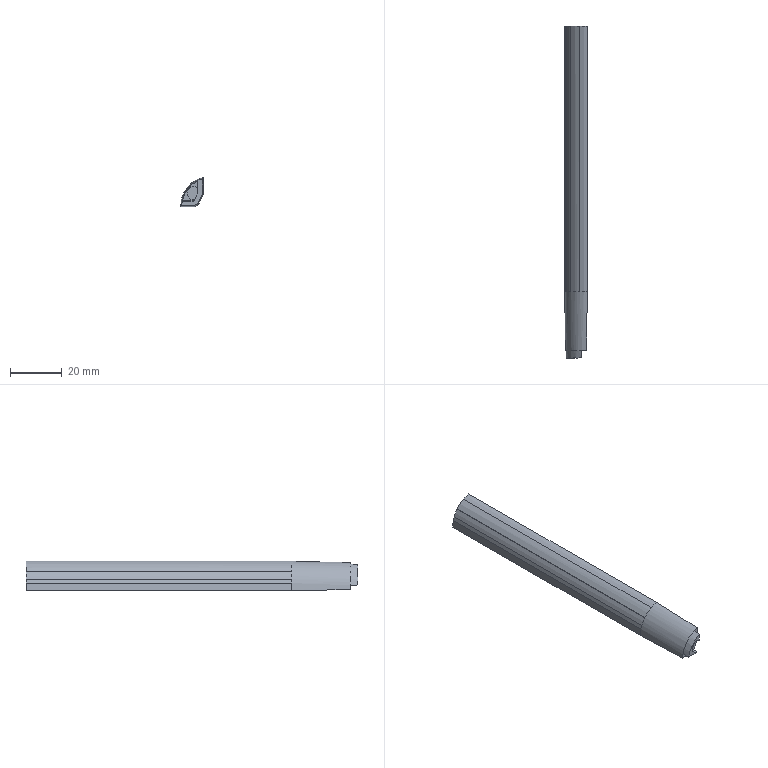Part | STEP file | 1 solid | 30 faces | box 8.776 x 127.988 x 11.283 mm | volume 8417 mm3 | plane 14 | spline 11 | cylinder 5 | commonest cylinder face diameters 5.025 x3 4.824 x2